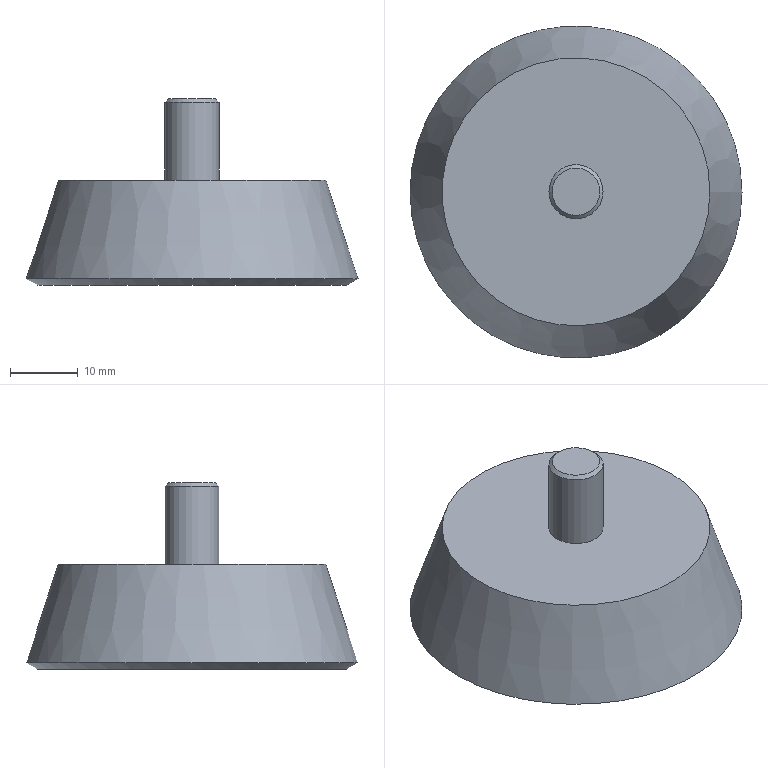Part | STEP file | 7100103W | 1 solid | 7 faces | box 48.954 x 48.954 x 27.5 mm | volume 24706 mm3 | plane 3 | cone 3 | cylinder 1 | commonest cylinder face diameters 8 x1
STEP:
#1=CARTESIAN_POINT('',(0.,0.,0.));
#2=DIRECTION('',(0.,0.,1.));
#3=DIRECTION('',(1.,0.,0.));
#4=AXIS2_PLACEMENT_3D('',#1,#2,#3);
#5=CARTESIAN_POINT('',(19.75,0.,0.));
#6=VERTEX_POINT('',#5);
#7=CARTESIAN_POINT('',(0.,0.,0.));
#8=DIRECTION('',(0.,0.,1.));
#9=DIRECTION('',(1.,0.,0.));
#10=AXIS2_PLACEMENT_3D('',#7,#8,#9);
#11=CIRCLE('',#10,19.75);
#12=CARTESIAN_POINT('',(0.,0.,0.));
#13=DIRECTION('',(0.,0.,1.));
#14=DIRECTION('',(1.,0.,0.));
#15=AXIS2_PLACEMENT_3D('',#12,#13,#14);
#16=PLANE('',#15);
#17=CARTESIAN_POINT('',(0.,0.));
#18=DIRECTION('',(1.,0.));
#19=AXIS2_PLACEMENT_2D('',#17,#18);
#20=CIRCLE('',#19,19.75);
#21=(GEOMETRIC_REPRESENTATION_CONTEXT(2)PARAMETRIC_REPRESENTATION_CONTEXT()REPRESENTATION_CONTEXT('',''));
#22=DEFINITIONAL_REPRESENTATION('',(#20),#21);
#23=PCURVE('',#16,#22);
#24=CARTESIAN_POINT('',(0.,0.,0.));
#25=DIRECTION('',(0.,0.,-1.));
#26=DIRECTION('',(1.,0.,0.));
#27=AXIS2_PLACEMENT_3D('',#24,#25,#26);
#28=CONICAL_SURFACE('',#27,19.75,0.3142);
#29=CARTESIAN_POINT('',(6.283,0.));
#30=DIRECTION('',(-1.,0.));
#31=VECTOR('',#30,1.);
#32=LINE('',#29,#31);
#33=(GEOMETRIC_REPRESENTATION_CONTEXT(2)PARAMETRIC_REPRESENTATION_CONTEXT()REPRESENTATION_CONTEXT('',''));
#34=DEFINITIONAL_REPRESENTATION('',(#32),#33);
#35=PCURVE('',#28,#34);
#36=SURFACE_CURVE('',#11,(#23,#35),.PCURVE_S1.);
#37=EDGE_CURVE('',#6,#6,#36,.T.);
#38=ORIENTED_EDGE('',*,*,#37,.T.);
#39=EDGE_LOOP('',(#38));
#40=FACE_BOUND('',#39,.T.);
#41=CARTESIAN_POINT('',(4.,0.,0.));
#42=VERTEX_POINT('',#41);
#43=CARTESIAN_POINT('',(0.,0.,0.));
#44=DIRECTION('',(0.,0.,1.));
#45=DIRECTION('',(1.,0.,0.));
#46=AXIS2_PLACEMENT_3D('',#43,#44,#45);
#47=CIRCLE('',#46,4.);
#48=CARTESIAN_POINT('',(0.,0.));
#49=DIRECTION('',(1.,0.));
#50=AXIS2_PLACEMENT_2D('',#48,#49);
#51=CIRCLE('',#50,4.);
#52=(GEOMETRIC_REPRESENTATION_CONTEXT(2)PARAMETRIC_REPRESENTATION_CONTEXT()REPRESENTATION_CONTEXT('',''));
#53=DEFINITIONAL_REPRESENTATION('',(#51),#52);
#54=PCURVE('',#16,#53);
#55=CARTESIAN_POINT('',(0.,0.,12.));
#56=DIRECTION('',(0.,0.,-1.));
#57=DIRECTION('',(-1.,0.,0.));
#58=AXIS2_PLACEMENT_3D('',#55,#56,#57);
#59=CYLINDRICAL_SURFACE('',#58,4.);
#60=CARTESIAN_POINT('',(9.425,12.));
#61=DIRECTION('',(-1.,0.));
#62=VECTOR('',#61,1.);
#63=LINE('',#60,#62);
#64=(GEOMETRIC_REPRESENTATION_CONTEXT(2)PARAMETRIC_REPRESENTATION_CONTEXT()REPRESENTATION_CONTEXT('',''));
#65=DEFINITIONAL_REPRESENTATION('',(#63),#64);
#66=PCURVE('',#59,#65);
#67=SURFACE_CURVE('',#47,(#54,#66),.PCURVE_S1.);
#68=EDGE_CURVE('',#42,#42,#67,.T.);
#69=ORIENTED_EDGE('',*,*,#68,.F.);
#70=EDGE_LOOP('',(#69));
#71=FACE_BOUND('',#70,.T.);
#72=ADVANCED_FACE('',(#40,#71),#16,.T.);
#73=CARTESIAN_POINT('',(-24.477,0.,-14.549));
#74=VERTEX_POINT('',#73);
#75=CARTESIAN_POINT('',(24.477,0.,-14.549));
#76=VERTEX_POINT('',#75);
#77=CARTESIAN_POINT('',(0.,0.,-14.549));
#78=DIRECTION('',(0.,0.,1.));
#79=DIRECTION('',(-1.,0.,0.));
#80=AXIS2_PLACEMENT_3D('',#77,#78,#79);
#81=CIRCLE('',#80,24.477);
#82=CARTESIAN_POINT('',(3.142,14.549));
#83=DIRECTION('',(-1.,0.));
#84=VECTOR('',#83,1.);
#85=LINE('',#82,#84);
#86=(GEOMETRIC_REPRESENTATION_CONTEXT(2)PARAMETRIC_REPRESENTATION_CONTEXT()REPRESENTATION_CONTEXT('',''));
#87=DEFINITIONAL_REPRESENTATION('',(#85),#86);
#88=PCURVE('',#28,#87);
#89=CARTESIAN_POINT('',(0.,0.,-14.549));
#90=DIRECTION('',(0.,0.,1.));
#91=DIRECTION('',(1.,0.,0.));
#92=AXIS2_PLACEMENT_3D('',#89,#90,#91);
#93=CONICAL_SURFACE('',#92,24.477,1.058);
#94=CARTESIAN_POINT('',(3.142,0.));
#95=DIRECTION('',(1.,0.));
#96=VECTOR('',#95,1.);
#97=LINE('',#94,#96);
#98=(GEOMETRIC_REPRESENTATION_CONTEXT(2)PARAMETRIC_REPRESENTATION_CONTEXT()REPRESENTATION_CONTEXT('',''));
#99=DEFINITIONAL_REPRESENTATION('',(#97),#98);
#100=PCURVE('',#93,#99);
#101=SURFACE_CURVE('',#81,(#88,#100),.PCURVE_S1.);
#102=EDGE_CURVE('',#74,#76,#101,.T.);
#103=ORIENTED_EDGE('',*,*,#102,.T.);
#104=CARTESIAN_POINT('',(19.75,0.,0.));
#105=CARTESIAN_POINT('',(24.477,0.,-14.549));
#106=B_SPLINE_CURVE_WITH_KNOTS('',1,(#104,#105),.UNSPECIFIED.,.F.,.F.,(2,2),(0.,15.298),.PIECEWISE_BEZIER_KNOTS.);
#107=CARTESIAN_POINT('',(0.,0.));
#108=DIRECTION('',(0.,1.));
#109=VECTOR('',#108,1.);
#110=LINE('',#107,#109);
#111=(GEOMETRIC_REPRESENTATION_CONTEXT(2)PARAMETRIC_REPRESENTATION_CONTEXT()REPRESENTATION_CONTEXT('',''));
#112=DEFINITIONAL_REPRESENTATION('',(#110),#111);
#113=PCURVE('',#28,#112);
#114=CARTESIAN_POINT('',(6.283,0.));
#115=DIRECTION('',(0.,1.));
#116=VECTOR('',#115,1.);
#117=LINE('',#114,#116);
#118=(GEOMETRIC_REPRESENTATION_CONTEXT(2)PARAMETRIC_REPRESENTATION_CONTEXT()REPRESENTATION_CONTEXT('',''));
#119=DEFINITIONAL_REPRESENTATION('',(#117),#118);
#120=PCURVE('',#28,#119);
#121=SEAM_CURVE('',#106,(#113,#120),.PCURVE_S1.);
#122=EDGE_CURVE('',#6,#76,#121,.T.);
#123=ORIENTED_EDGE('',*,*,#122,.F.);
#124=ORIENTED_EDGE('',*,*,#37,.F.);
#125=ORIENTED_EDGE('',*,*,#122,.T.);
#126=CARTESIAN_POINT('',(0.,0.,-14.549));
#127=DIRECTION('',(0.,0.,1.));
#128=DIRECTION('',(-1.,0.,0.));
#129=AXIS2_PLACEMENT_3D('',#126,#127,#128);
#130=CIRCLE('',#129,24.477);
#131=CARTESIAN_POINT('',(9.425,14.549));
#132=DIRECTION('',(-1.,0.));
#133=VECTOR('',#132,1.);
#134=LINE('',#131,#133);
#135=(GEOMETRIC_REPRESENTATION_CONTEXT(2)PARAMETRIC_REPRESENTATION_CONTEXT()REPRESENTATION_CONTEXT('',''));
#136=DEFINITIONAL_REPRESENTATION('',(#134),#135);
#137=PCURVE('',#28,#136);
#138=CARTESIAN_POINT('',(-3.142,0.));
#139=DIRECTION('',(1.,0.));
#140=VECTOR('',#139,1.);
#141=LINE('',#138,#140);
#142=(GEOMETRIC_REPRESENTATION_CONTEXT(2)PARAMETRIC_REPRESENTATION_CONTEXT()REPRESENTATION_CONTEXT('',''));
#143=DEFINITIONAL_REPRESENTATION('',(#141),#142);
#144=PCURVE('',#93,#143);
#145=SURFACE_CURVE('',#130,(#137,#144),.PCURVE_S1.);
#146=EDGE_CURVE('',#76,#74,#145,.T.);
#147=ORIENTED_EDGE('',*,*,#146,.T.);
#148=EDGE_LOOP('',(#103,#123,#124,#125,#147));
#149=FACE_BOUND('',#148,.T.);
#150=ADVANCED_FACE('',(#149),#28,.T.);
#151=CARTESIAN_POINT('',(22.786,0.,-15.5));
#152=VERTEX_POINT('',#151);
#153=CARTESIAN_POINT('',(0.,0.,-15.5));
#154=DIRECTION('',(0.,0.,-1.));
#155=DIRECTION('',(1.,0.,0.));
#156=AXIS2_PLACEMENT_3D('',#153,#154,#155);
#157=CIRCLE('',#156,22.786);
#158=CARTESIAN_POINT('',(0.,0.,-15.5));
#159=DIRECTION('',(0.,0.,1.));
#160=DIRECTION('',(1.,0.,0.));
#161=AXIS2_PLACEMENT_3D('',#158,#159,#160);
#162=PLANE('',#161);
#163=CARTESIAN_POINT('',(22.786,0.));
#164=CARTESIAN_POINT('',(22.786,-39.467));
#165=CARTESIAN_POINT('',(-11.393,-19.733));
#166=CARTESIAN_POINT('',(-45.573,0.));
#167=CARTESIAN_POINT('',(-11.393,19.733));
#168=CARTESIAN_POINT('',(22.786,39.467));
#169=CARTESIAN_POINT('',(22.786,0.));
#170=(BOUNDED_CURVE()B_SPLINE_CURVE(2,(#163,#164,#165,#166,#167,#168,#169),.UNSPECIFIED.,.T.,.F.)B_SPLINE_CURVE_WITH_KNOTS((1,2,2,2,2,1),(-2.094,0.,2.094,4.189,6.283,8.378),.UNSPECIFIED.)CURVE()GEOMETRIC_REPRESENTATION_ITEM()RATIONAL_B_SPLINE_CURVE((1.,0.5,1.,0.5,1.,0.5,1.))REPRESENTATION_ITEM(''));
#171=(GEOMETRIC_REPRESENTATION_CONTEXT(2)PARAMETRIC_REPRESENTATION_CONTEXT()REPRESENTATION_CONTEXT('',''));
#172=DEFINITIONAL_REPRESENTATION('',(#170),#171);
#173=PCURVE('',#162,#172);
#174=CARTESIAN_POINT('',(6.283,-0.9511));
#175=DIRECTION('',(-1.,0.));
#176=VECTOR('',#175,1.);
#177=LINE('',#174,#176);
#178=(GEOMETRIC_REPRESENTATION_CONTEXT(2)PARAMETRIC_REPRESENTATION_CONTEXT()REPRESENTATION_CONTEXT('',''));
#179=DEFINITIONAL_REPRESENTATION('',(#177),#178);
#180=PCURVE('',#93,#179);
#181=SURFACE_CURVE('',#157,(#173,#180),.PCURVE_S1.);
#182=EDGE_CURVE('',#152,#152,#181,.T.);
#183=ORIENTED_EDGE('',*,*,#182,.T.);
#184=EDGE_LOOP('',(#183));
#185=FACE_BOUND('',#184,.T.);
#186=ADVANCED_FACE('',(#185),#162,.F.);
#187=ORIENTED_EDGE('',*,*,#182,.F.);
#188=CARTESIAN_POINT('',(22.786,0.,-15.5));
#189=CARTESIAN_POINT('',(24.477,0.,-14.549));
#190=B_SPLINE_CURVE_WITH_KNOTS('',1,(#188,#189),.UNSPECIFIED.,.F.,.F.,(2,2),(-1.94,0.),.PIECEWISE_BEZIER_KNOTS.);
#191=CARTESIAN_POINT('',(6.283,0.));
#192=DIRECTION('',(0.,1.));
#193=VECTOR('',#192,1.);
#194=LINE('',#191,#193);
#195=(GEOMETRIC_REPRESENTATION_CONTEXT(2)PARAMETRIC_REPRESENTATION_CONTEXT()REPRESENTATION_CONTEXT('',''));
#196=DEFINITIONAL_REPRESENTATION('',(#194),#195);
#197=PCURVE('',#93,#196);
#198=CARTESIAN_POINT('',(0.,0.));
#199=DIRECTION('',(0.,1.));
#200=VECTOR('',#199,1.);
#201=LINE('',#198,#200);
#202=(GEOMETRIC_REPRESENTATION_CONTEXT(2)PARAMETRIC_REPRESENTATION_CONTEXT()REPRESENTATION_CONTEXT('',''));
#203=DEFINITIONAL_REPRESENTATION('',(#201),#202);
#204=PCURVE('',#93,#203);
#205=SEAM_CURVE('',#190,(#197,#204),.PCURVE_S1.);
#206=EDGE_CURVE('',#152,#76,#205,.T.);
#207=ORIENTED_EDGE('',*,*,#206,.T.);
#208=ORIENTED_EDGE('',*,*,#102,.F.);
#209=ORIENTED_EDGE('',*,*,#146,.F.);
#210=ORIENTED_EDGE('',*,*,#206,.F.);
#211=EDGE_LOOP('',(#187,#207,#208,#209,#210));
#212=FACE_BOUND('',#211,.T.);
#213=ADVANCED_FACE('',(#212),#93,.T.);
#214=CARTESIAN_POINT('',(4.,0.,11.5));
#215=VERTEX_POINT('',#214);
#216=CARTESIAN_POINT('',(0.,0.,11.5));
#217=DIRECTION('',(0.,0.,-1.));
#218=DIRECTION('',(1.,0.,0.));
#219=AXIS2_PLACEMENT_3D('',#216,#217,#218);
#220=CIRCLE('',#219,4.);
#221=CARTESIAN_POINT('',(3.142,0.5));
#222=DIRECTION('',(1.,0.));
#223=VECTOR('',#222,1.);
#224=LINE('',#221,#223);
#225=(GEOMETRIC_REPRESENTATION_CONTEXT(2)PARAMETRIC_REPRESENTATION_CONTEXT()REPRESENTATION_CONTEXT('',''));
#226=DEFINITIONAL_REPRESENTATION('',(#224),#225);
#227=PCURVE('',#59,#226);
#228=CARTESIAN_POINT('',(0.,0.,12.));
#229=DIRECTION('',(0.,0.,-1.));
#230=DIRECTION('',(-1.,0.,0.));
#231=AXIS2_PLACEMENT_3D('',#228,#229,#230);
#232=CONICAL_SURFACE('',#231,3.5,0.7854);
#233=CARTESIAN_POINT('',(3.142,0.5));
#234=DIRECTION('',(1.,0.));
#235=VECTOR('',#234,1.);
#236=LINE('',#233,#235);
#237=(GEOMETRIC_REPRESENTATION_CONTEXT(2)PARAMETRIC_REPRESENTATION_CONTEXT()REPRESENTATION_CONTEXT('',''));
#238=DEFINITIONAL_REPRESENTATION('',(#236),#237);
#239=PCURVE('',#232,#238);
#240=SURFACE_CURVE('',#220,(#227,#239),.PCURVE_S1.);
#241=EDGE_CURVE('',#215,#215,#240,.T.);
#242=ORIENTED_EDGE('',*,*,#241,.T.);
#243=CARTESIAN_POINT('',(4.,0.,11.5));
#244=CARTESIAN_POINT('',(4.,0.,0.));
#245=B_SPLINE_CURVE_WITH_KNOTS('',1,(#243,#244),.UNSPECIFIED.,.F.,.F.,(2,2),(0.5,12.),.PIECEWISE_BEZIER_KNOTS.);
#246=CARTESIAN_POINT('',(9.425,0.));
#247=DIRECTION('',(0.,1.));
#248=VECTOR('',#247,1.);
#249=LINE('',#246,#248);
#250=(GEOMETRIC_REPRESENTATION_CONTEXT(2)PARAMETRIC_REPRESENTATION_CONTEXT()REPRESENTATION_CONTEXT('',''));
#251=DEFINITIONAL_REPRESENTATION('',(#249),#250);
#252=PCURVE('',#59,#251);
#253=CARTESIAN_POINT('',(3.142,0.));
#254=DIRECTION('',(0.,1.));
#255=VECTOR('',#254,1.);
#256=LINE('',#253,#255);
#257=(GEOMETRIC_REPRESENTATION_CONTEXT(2)PARAMETRIC_REPRESENTATION_CONTEXT()REPRESENTATION_CONTEXT('',''));
#258=DEFINITIONAL_REPRESENTATION('',(#256),#257);
#259=PCURVE('',#59,#258);
#260=SEAM_CURVE('',#245,(#252,#259),.PCURVE_S1.);
#261=EDGE_CURVE('',#215,#42,#260,.T.);
#262=ORIENTED_EDGE('',*,*,#261,.T.);
#263=ORIENTED_EDGE('',*,*,#68,.T.);
#264=ORIENTED_EDGE('',*,*,#261,.F.);
#265=EDGE_LOOP('',(#242,#262,#263,#264));
#266=FACE_BOUND('',#265,.T.);
#267=ADVANCED_FACE('',(#266),#59,.T.);
#268=CARTESIAN_POINT('',(3.5,0.,12.));
#269=VERTEX_POINT('',#268);
#270=CARTESIAN_POINT('',(0.,0.,12.));
#271=DIRECTION('',(0.,0.,1.));
#272=DIRECTION('',(1.,0.,0.));
#273=AXIS2_PLACEMENT_3D('',#270,#271,#272);
#274=CIRCLE('',#273,3.5);
#275=CARTESIAN_POINT('',(0.,0.,12.));
#276=DIRECTION('',(0.,0.,1.));
#277=DIRECTION('',(1.,0.,0.));
#278=AXIS2_PLACEMENT_3D('',#275,#276,#277);
#279=PLANE('',#278);
#280=CARTESIAN_POINT('',(0.,0.));
#281=DIRECTION('',(1.,0.));
#282=AXIS2_PLACEMENT_2D('',#280,#281);
#283=CIRCLE('',#282,3.5);
#284=(GEOMETRIC_REPRESENTATION_CONTEXT(2)PARAMETRIC_REPRESENTATION_CONTEXT()REPRESENTATION_CONTEXT('',''));
#285=DEFINITIONAL_REPRESENTATION('',(#283),#284);
#286=PCURVE('',#279,#285);
#287=CARTESIAN_POINT('',(9.425,0.));
#288=DIRECTION('',(-1.,0.));
#289=VECTOR('',#288,1.);
#290=LINE('',#287,#289);
#291=(GEOMETRIC_REPRESENTATION_CONTEXT(2)PARAMETRIC_REPRESENTATION_CONTEXT()REPRESENTATION_CONTEXT('',''));
#292=DEFINITIONAL_REPRESENTATION('',(#290),#291);
#293=PCURVE('',#232,#292);
#294=SURFACE_CURVE('',#274,(#286,#293),.PCURVE_S1.);
#295=EDGE_CURVE('',#269,#269,#294,.T.);
#296=ORIENTED_EDGE('',*,*,#295,.T.);
#297=EDGE_LOOP('',(#296));
#298=FACE_BOUND('',#297,.T.);
#299=ADVANCED_FACE('',(#298),#279,.T.);
#300=ORIENTED_EDGE('',*,*,#241,.F.);
#301=CARTESIAN_POINT('',(3.5,0.,12.));
#302=CARTESIAN_POINT('',(4.,0.,11.5));
#303=B_SPLINE_CURVE_WITH_KNOTS('',1,(#301,#302),.UNSPECIFIED.,.F.,.F.,(2,2),(0.,0.7071),.PIECEWISE_BEZIER_KNOTS.);
#304=CARTESIAN_POINT('',(3.142,0.));
#305=DIRECTION('',(0.,1.));
#306=VECTOR('',#305,1.);
#307=LINE('',#304,#306);
#308=(GEOMETRIC_REPRESENTATION_CONTEXT(2)PARAMETRIC_REPRESENTATION_CONTEXT()REPRESENTATION_CONTEXT('',''));
#309=DEFINITIONAL_REPRESENTATION('',(#307),#308);
#310=PCURVE('',#232,#309);
#311=CARTESIAN_POINT('',(9.425,0.));
#312=DIRECTION('',(0.,1.));
#313=VECTOR('',#312,1.);
#314=LINE('',#311,#313);
#315=(GEOMETRIC_REPRESENTATION_CONTEXT(2)PARAMETRIC_REPRESENTATION_CONTEXT()REPRESENTATION_CONTEXT('',''));
#316=DEFINITIONAL_REPRESENTATION('',(#314),#315);
#317=PCURVE('',#232,#316);
#318=SEAM_CURVE('',#303,(#310,#317),.PCURVE_S1.);
#319=EDGE_CURVE('',#269,#215,#318,.T.);
#320=ORIENTED_EDGE('',*,*,#319,.F.);
#321=ORIENTED_EDGE('',*,*,#295,.F.);
#322=ORIENTED_EDGE('',*,*,#319,.T.);
#323=EDGE_LOOP('',(#300,#320,#321,#322));
#324=FACE_BOUND('',#323,.T.);
#325=ADVANCED_FACE('',(#324),#232,.T.);
#326=CLOSED_SHELL('',(#72,#150,#186,#213,#267,#299,#325));
#327=MANIFOLD_SOLID_BREP('',#326);
#328=(LENGTH_UNIT()NAMED_UNIT(*)SI_UNIT(.MILLI.,.METRE.));
#329=UNCERTAINTY_MEASURE_WITH_UNIT(LENGTH_MEASURE(0.000005),#328,'','');
#330=(NAMED_UNIT(*)PLANE_ANGLE_UNIT()SI_UNIT($,.RADIAN.));
#331=(NAMED_UNIT(*)SI_UNIT($,.STERADIAN.)SOLID_ANGLE_UNIT());
#332=(GEOMETRIC_REPRESENTATION_CONTEXT(3)GLOBAL_UNCERTAINTY_ASSIGNED_CONTEXT((#329))GLOBAL_UNIT_ASSIGNED_CONTEXT((#328,#330,#331))REPRESENTATION_CONTEXT('',''));
#333=ADVANCED_BREP_SHAPE_REPRESENTATION('',(#4,#327),#332);